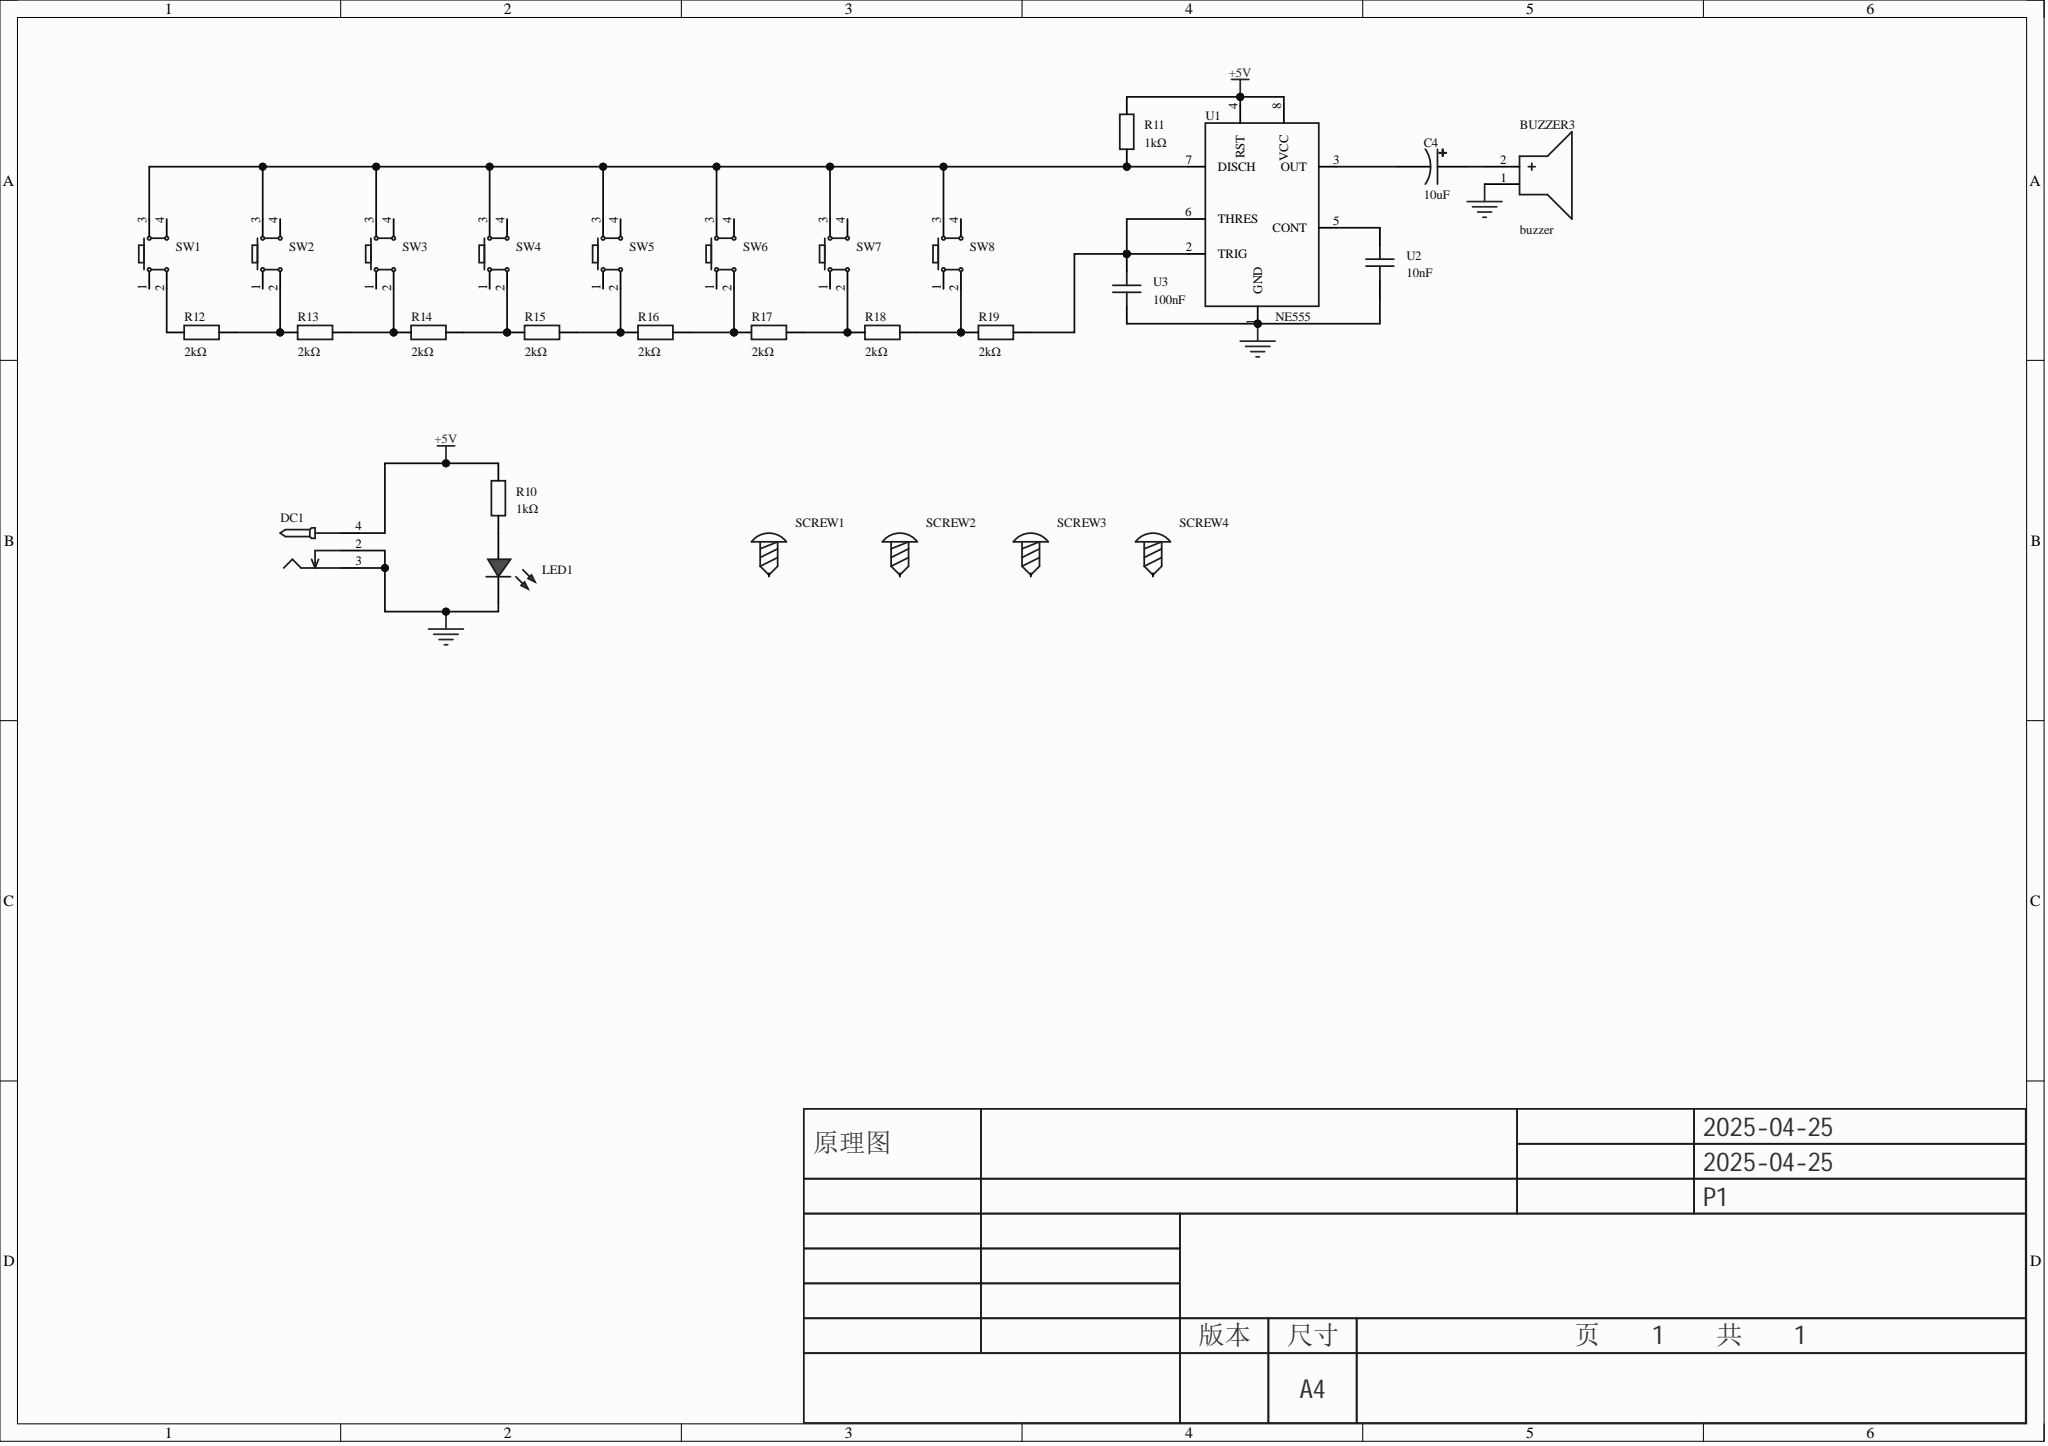Circuit board | Altium Designer | 29 parts | 16 nets
Bill of materials:
Comment,Description,Designator,Footprint,LibRef,Quantity
"buzzer","","BUZZER3","BUZ-TH_BD12.0-P6.00-D0.9-RD","buzzer","1"
"10uF","容值:4.7uF;精度:±20%;额定电压:100V;","C4","CAP-TH_BD5.0-P2.00-D0.8-FD","KM475M100D11RR0VH2FP0","1"
"","","DC1","DC-2.0","DC-005_2.0","1"
"","","LED1","LED_TH-3mm","LED_TH-R_3mm","1"
"1kΩ","","R10, R11","Res_1/8W","Res_AXIAL-1/8W","2"
"2kΩ","","R12, R13, R14, R15, R16, R17, R18, R19","Res_1/8W","Res_AXIAL-1/8W","8"
"","","SCREW1, SCREW2, SCREW3, SCREW4","M3螺丝","M3螺丝","4"
"","","SW1, SW2, SW3, SW4, SW5, SW6, SW7, SW8","SW-TH_4P-L6.0-W6.0-P4.50-LS6.5","Key_TH_6x6x6","8"
"NE555","NE555 单精度定时器","U1","PDIP-8_L9.6-W6.4-P2.54-LS7.9-BL-1","NE555PE4","1"
"10nF","容值:10nF;精度:±10%;额定电压:50V;温度系数:X7R;","U2","CAP-TH_L4.0-W2.5-P2.50-D0.5","FK18X7R1H103K","1"
"100nF","容值:10nF;精度:±10%;额定电压:50V;温度系数:X7R;","U3","CAP-TH_L4.0-W2.5-P2.50-D0.5","FK18X7R1H103K","1"
Netlist (Protel format):
[
BUZZER3
BUZ-TH_BD12.0-P6.00-D0.9-RD
buzzer



]
[
C4
CAP-TH_BD5.0-P2.00-D0.8-FD
10uF



]
[
DC1
DC-2.0




]
[
LED1
LED_TH-3mm




]
[
R10
Res_1/8W
1kΩ



]
[
R11
Res_1/8W
1kΩ



]
[
R12
Res_1/8W
2kΩ



]
[
R13
Res_1/8W
2kΩ



]
[
R14
Res_1/8W
2kΩ



]
[
R15
Res_1/8W
2kΩ



]
[
R16
Res_1/8W
2kΩ



]
[
R17
Res_1/8W
2kΩ



]
[
R18
Res_1/8W
2kΩ



]
[
R19
Res_1/8W
2kΩ



]
[
SCREW1
M3螺丝




]
[
SCREW2
M3螺丝




]
[
SCREW3
M3螺丝




]
[
SCREW4
M3螺丝




]
[
SW1
SW-TH_4P-L6.0-W6.0-P4.50-LS6.5




]
[
SW2
SW-TH_4P-L6.0-W6.0-P4.50-LS6.5




]
[
SW3
SW-TH_4P-L6.0-W6.0-P4.50-LS6.5




]
[
SW4
SW-TH_4P-L6.0-W6.0-P4.50-LS6.5




]
[
SW5
SW-TH_4P-L6.0-W6.0-P4.50-LS6.5




]
[
SW6
SW-TH_4P-L6.0-W6.0-P4.50-LS6.5




]
[
SW7
SW-TH_4P-L6.0-W6.0-P4.50-LS6.5




]
[
SW8
SW-TH_4P-L6.0-W6.0-P4.50-LS6.5




]
[
U1
PDIP-8_L9.6-W6.4-P2.54-LS7.9-BL-1
NE555



]
[
U2
CAP-TH_L4.0-W2.5-P2.50-D0.5
10nF



]
[
U3
CAP-TH_L4.0-W2.5-P2.50-D0.5
100nF



]
(
NetU1_5
U1-5
U2-2
)
(
NetR19_2
R19-2
U1-2
U1-6
U3-2
)
(
NetR18_2
R18-2
R19-1
SW8-2
)
(
NetR17_2
R17-2
R18-1
SW7-2
)
(
NetR16_2
R16-2
R17-1
SW6-2
)
(
NetR15_2
R15-2
R16-1
SW5-2
)
(
NetR14_2
R14-2
R15-1
SW4-2
)
(
NetR13_2
R13-2
R14-1
SW3-2
)
(
NetR12_2
R12-2
R13-1
SW2-2
)
(
NetR12_1
R12-1
SW1-2
)
(
NetR11_1
R11-1
SW1-3
SW2-3
SW3-3
SW4-3
SW5-3
SW6-3
SW7-3
SW8-3
U1-7
)
(
NetLED1_1
LED1-1
R10-1
)
(
NetC4_2
C4-2
U1-3
)
(
NetBUZZER3_2
BUZZER3-2
C4-1
)
(
GND
BUZZER3-1
DC1-2
DC1-3
LED1-2
U1-1
U2-1
U3-1
)
(
+5V
DC1-4
R10-2
R11-2
U1-4
U1-8
)